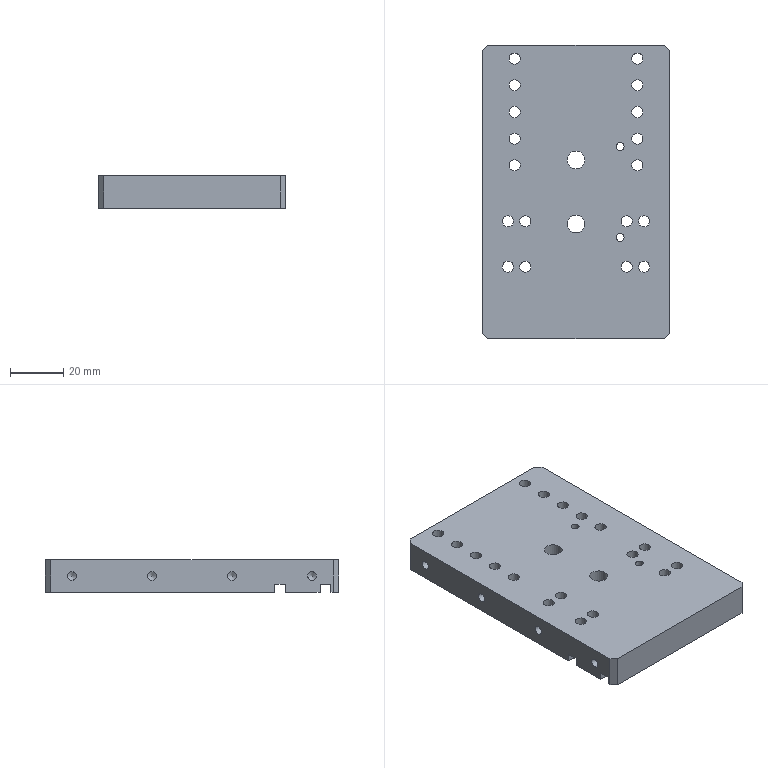Part | 1 solid | 60 faces | box 70 x 110 x 12 mm | volume 85149 mm3 | cylinder 32 | plane 20 | cone 8 | commonest cylinder face diameters 4.2 x18 3.3 x8 3 x2 6.6 x2 11 x2